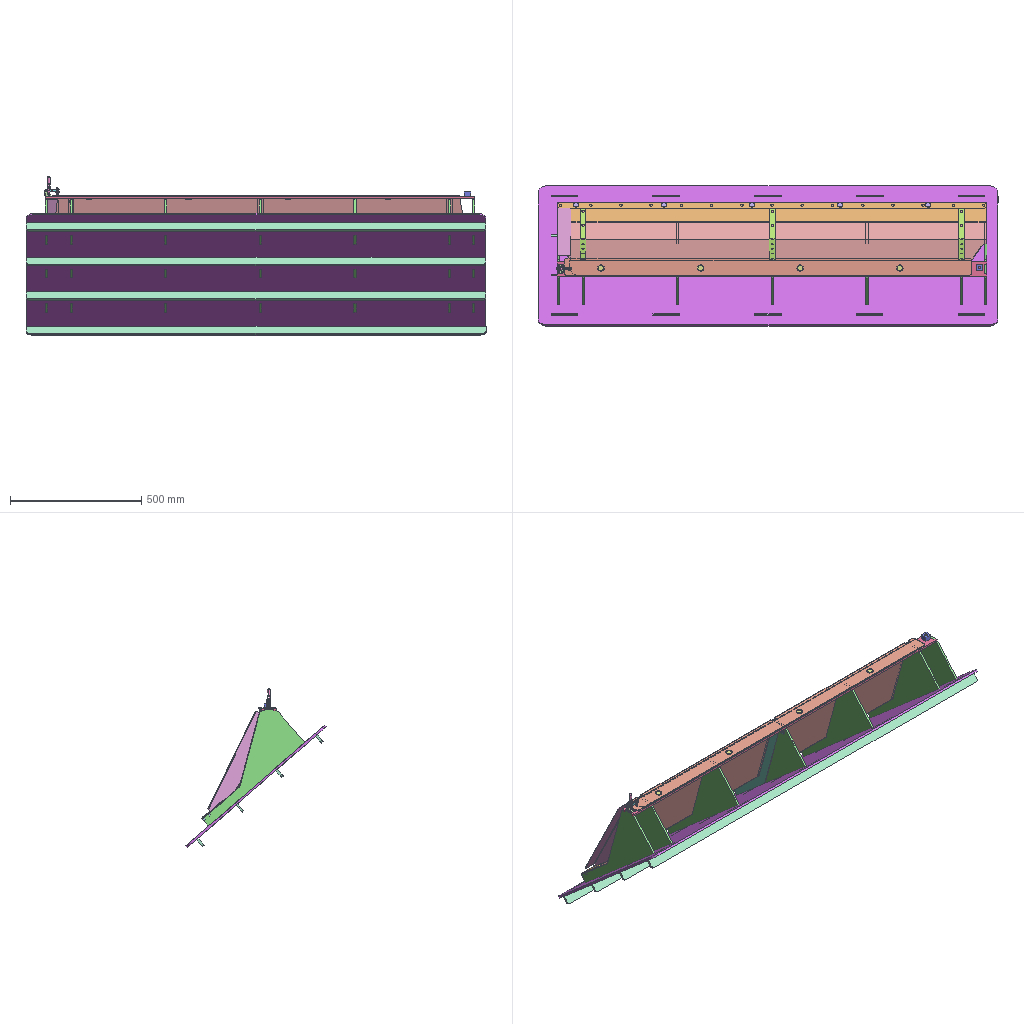Assembly | SolidWorks | 16 different items | 34 placed | box 1750 x 534 x 605 mm
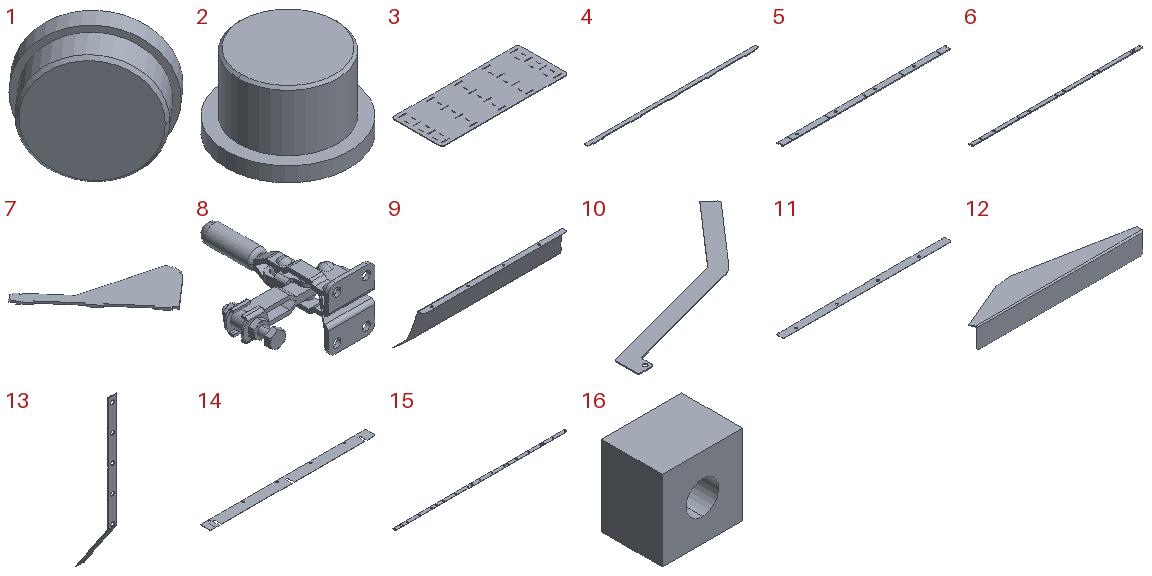Parts list (item | quantity | size | volume | features):
1 | x5 | 18.175 x 19.26 x 20 mm | 2208 mm3 | features Chamfer 1, Revolution 1
2 | x4 | 25 x 25 x 15 mm | 5235 mm3 | features Chamfer 1, Revolution 1
3 | x1 | 1750 x 700 x 8 mm | 9598619 mm3 | features FlatPattern 1, SMBaseFlange 1, SheetMetal 1
4 | x4 | 1750 x 42.5 x 8 mm | 519657 mm3 | features FlatPattern 1, SMBaseFlange 1, SheetMetal 1
5 | x1 | 1635 x 55 x 8 mm | 693667 mm3 | features FlatPattern 1, SMBaseFlange 1, SheetMetal 1
6 | x1 | 1635 x 34.8 x 8 mm | 435932 mm3 | features FlatPattern 1, SMBaseFlange 1, SheetMetal 1
7 | x7 | 445.432 x 383.748 x 8 mm | 369427 mm3 | features FlatPattern 1, SMBaseFlange 1, SheetMetal 1
8 | x1 | 56.45 x 77.62 x 33.3 mm | 10418 mm3 | features BaseBody 5
9 | x1 | 1635 x 277.618 x 421.117 mm | 1397928 mm3 | features SM3dBend 2, FlatPattern 1, SMBaseFlange 1, SheetMetal 1
10 | x1 | 443.878 x 276.569 x 2.3 mm | 42757 mm3 | features FlatPattern 1, SMBaseFlange 1, SheetMetal 1
11 | x1 | 1550 x 65 x 2.3 mm | 227708 mm3 | features FlatPattern 1, SMBaseFlange 1, SheetMetal 1
12 | x1 | 421 x 66.98 x 52 mm | 61109 mm3 | features Chamfer 1, Fillet 1, FlatPattern 1, ICE 1, SMBaseFlange 1, SheetMetal 1
13 | x3 | 22 x 88.001 x 431.5 mm | 15223 mm3 | features ICE 2, FlatPattern 1, SMBaseFlange 1, SheetMetal 1
14 | x1 | 1635 x 100 x 2.3 mm | 362359 mm3 | features FlatPattern 1, SMBaseFlange 1, SheetMetal 1
15 | x1 | 1630 x 30 x 1.6 mm | 74182 mm3 | features Fillet 1, FlatPattern 1, SMBaseFlange 1, SheetMetal 1
16 | x1 | 25 x 19 x 25 mm | 10322 mm3 | features Extrusion 1, HoleWzd 1
Mates (type | each side: item.copy, entity, surface, feature):
Coincident | 9.1 face plane Base-Flange1 | 15.1 face plane Base-Flange1
Concentric | 9.1 face cylinder Base-Flange1 | 15.1 face cylinder Base-Flange1 | 2 times
Coincident | 9.1 face plane Base-Flange1 | 13.1 face plane Base-Flange1 | 2 times
DistanceDim | 9.1 face plane Base-Flange1 | 13.1 face plane Base-Flange1
Coincident | 9.1 face plane Base-Flange1 | 12.1 face plane Base-Flange1
Coincident | 9.1 face plane Base-Flange1 | 12.1 face plane Cut-Extrude1 | 2 times
InPlace | 10.1 plane | assembly plane
InPlace | 9.1 face plane Base-Flange1 | 14.1 plane
InPlace | 1.1 plane | assembly plane
InPlace | 9.1 face plane Base-Flange1 | 7.1 plane
InPlace | 7.1 face plane Base-Flange1 | 5.1 plane
InPlace | 9.1 face plane Base-Flange1 | 6.1 plane
Concentric | 5.1 face cylinder Base-Flange1 | 2.1 face cylinder Revolve1
Coincident | 9.1 face plane Base-Flange1 | 2.1 face plane Revolve1
InPlace | 7.2 face plane Base-Flange1 | 3.1 plane
InPlace | 4.1 plane | assembly plane
InPlace | 9.1 face plane Base-Flange1 | 11.1 plane
Coincident | 5.1 face plane Base-Flange1 | 16.1 face plane Boss-Extrude1
DistanceDim | 5.1 face plane Base-Flange1 | 16.1 face plane Boss-Extrude1
DistanceDim | 16.1 face plane Boss-Extrude1 | 5.1 face plane Base-Flange1
Coincident | 5.1 face plane Base-Flange1 | 8.1 face plane TC1-1 vertical flange quick clamp [TCS1-1].step-1/_TCS1-1(seat).step-1-solid1
Coincident | 7.1 face plane Base-Flange1 | 8.1 face plane TC1-1 vertical flange quick clamp [TCS1-1].step-1/_TCS1-1(seat).step-1-solid1
DistanceDim | 8.1 face plane TC1-1 vertical flange quick clamp [TCS1-1].step-1/_TCS1-1(seat).step-1-solid1 | 5.1 face plane Base-Flange1